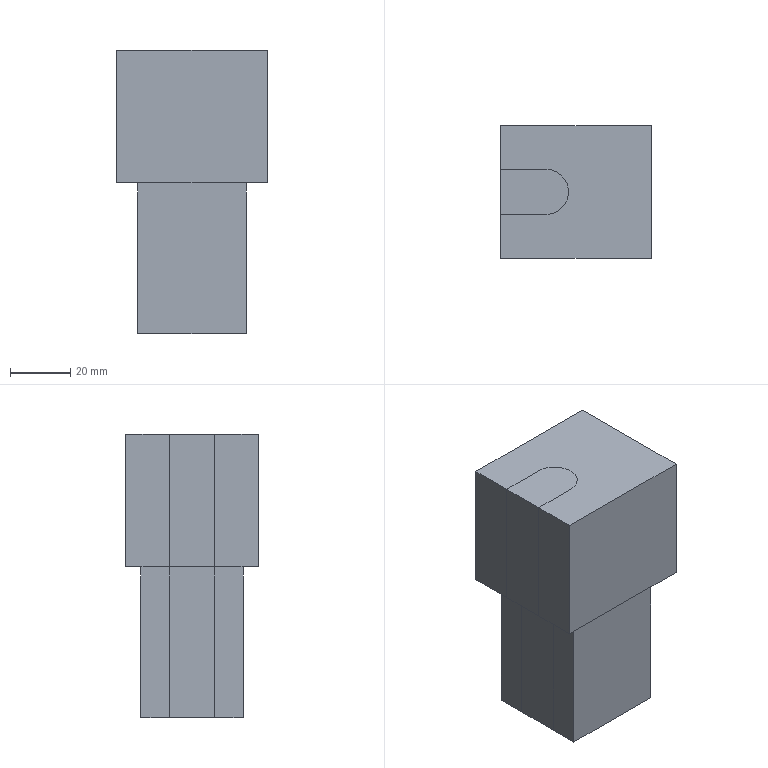Part | STEP file | 00000 | 2 solids | 24 faces | box 50 x 44 x 94 mm | volume 158000 mm3 | plane 22 | cylinder 2 | commonest cylinder face diameters 15 x2